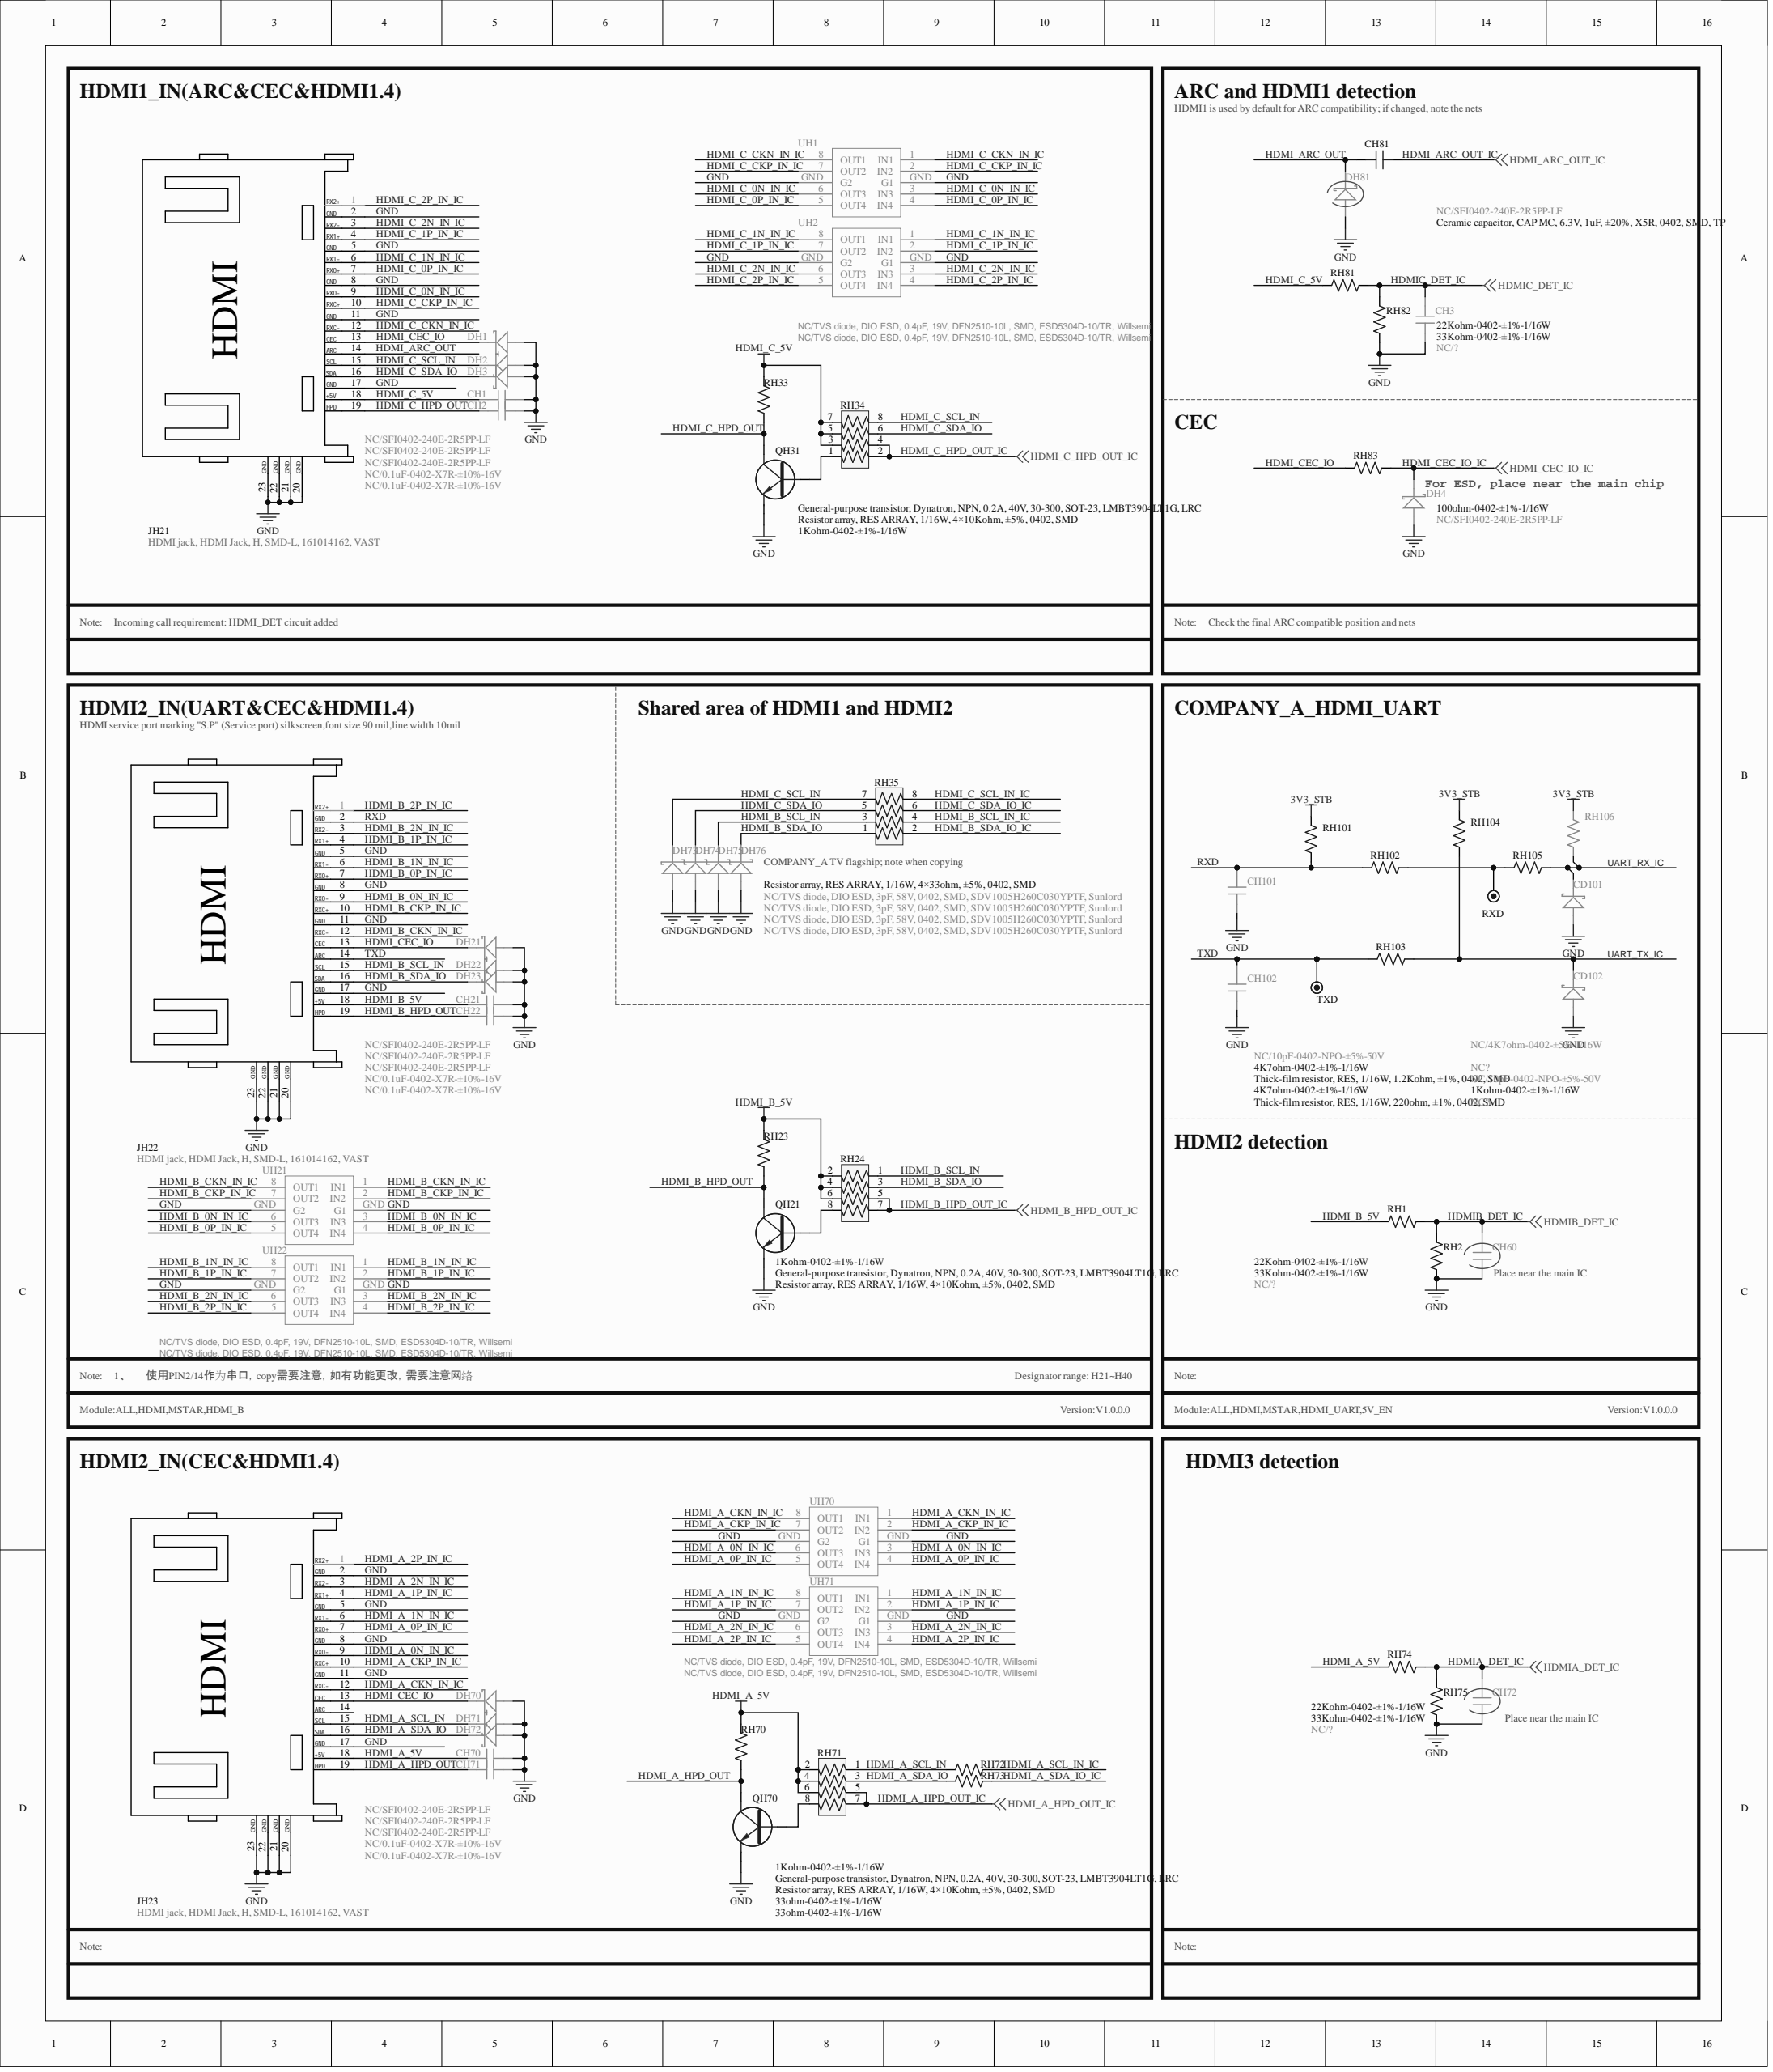Circuit board | Altium Designer | 541 parts | 263 nets | one sheet of the schematic
Parts on this sheet (reference | value | footprint):
CD101 | NC? | DIODE-S0402
CD102 | NC? | DIODE-S0402
CH1 | NC/0.1uF-0402-X7R-±10%-16V | C0402
CH2 | NC/0.1uF-0402-X7R-±10%-16V | C0402
CH3 | NC/? | C0402
CH21 | NC/0.1uF-0402-X7R-±10%-16V | C0402
CH22 | NC/0.1uF-0402-X7R-±10%-16V | C0402
CH60 | NC/? | C0402
CH70 | NC/0.1uF-0402-X7R-±10%-16V | C0402
CH71 | NC/0.1uF-0402-X7R-±10%-16V | C0402
CH72 | NC/? | C0402
CH81 | Ceramic capacitor, CAP MC, 6.3V, 1uF, ±20%, X5R, 0402, SMD, TP | C0402
CH101 | NC/10pF-0402-NPO-±5%-50V | C0402
CH102 | NC/10pF-0402-NPO-±5%-50V | C0402
DH1 | NC/SFI0402-240E-2R5PP-LF | DIODE-S0402
DH2 | NC/SFI0402-240E-2R5PP-LF | DIODE-S0402
DH3 | NC/SFI0402-240E-2R5PP-LF | DIODE-S0402
DH4 | NC/SFI0402-240E-2R5PP-LF | DIODE-S0402
DH21 | NC/SFI0402-240E-2R5PP-LF | DIODE-S0402
DH22 | NC/SFI0402-240E-2R5PP-LF | DIODE-S0402
DH23 | NC/SFI0402-240E-2R5PP-LF | DIODE-S0402
DH70 | NC/SFI0402-240E-2R5PP-LF | DIODE-S0402
DH71 | NC/SFI0402-240E-2R5PP-LF | DIODE-S0402
DH72 | NC/SFI0402-240E-2R5PP-LF | DIODE-S0402
DH73 | NC/TVS diode, DIO ESD, 3pF, 58V, 0402, SMD, SDV1005H260C030YPTF, Sunlord | DIODE-S0402
DH74 | NC/TVS diode, DIO ESD, 3pF, 58V, 0402, SMD, SDV1005H260C030YPTF, Sunlord | DIODE-S0402
DH75 | NC/TVS diode, DIO ESD, 3pF, 58V, 0402, SMD, SDV1005H260C030YPTF, Sunlord | DIODE-S0402
DH76 | NC/TVS diode, DIO ESD, 3pF, 58V, 0402, SMD, SDV1005H260C030YPTF, Sunlord | DIODE-S0402
DH81 | NC/SFI0402-240E-2R5PP-LF | DIODE-S0402
JH21 | HDMI jack, HDMI Jack, H, SMD-L, 161014162, VAST | HDMI-HS-1
JH22 | HDMI jack, HDMI Jack, H, SMD-L, 161014162, VAST | HDMI-HS-1
JH23 | HDMI jack, HDMI Jack, H, SMD-L, 161014162, VAST | HDMI-HS-1
QH21 | General-purpose transistor, Dynatron, NPN, 0.2A, 40V, 30-300, SOT-23, LMBT3904LT1G, LRC | SOT-23
QH31 | General-purpose transistor, Dynatron, NPN, 0.2A, 40V, 30-300, SOT-23, LMBT3904LT1G, LRC | SOT-23
QH70 | General-purpose transistor, Dynatron, NPN, 0.2A, 40V, 30-300, SOT-23, LMBT3904LT1G, LRC | SOT-23
RH1 | 22Kohm-0402-±1%-1/16W | R0402
RH2 | 33Kohm-0402-±1%-1/16W | R0402
RH23 | 1Kohm-0402-±1%-1/16W | R0402
RH24 | Resistor array, RES ARRAY, 1/16W, 4×10Kohm, ±5%, 0402, SMD | RA0402
RH33 | 1Kohm-0402-±1%-1/16W | R0402
RH34 | Resistor array, RES ARRAY, 1/16W, 4×10Kohm, ±5%, 0402, SMD | RA0402
RH35 | Resistor array, RES ARRAY, 1/16W, 4×33ohm, ±5%, 0402, SMD | RA0402
RH70 | 1Kohm-0402-±1%-1/16W | R0402
RH71 | Resistor array, RES ARRAY, 1/16W, 4×10Kohm, ±5%, 0402, SMD | RA0402
RH72 | 33ohm-0402-±1%-1/16W | R0402
RH73 | 33ohm-0402-±1%-1/16W | R0402
RH74 | 22Kohm-0402-±1%-1/16W | R0402
RH75 | 33Kohm-0402-±1%-1/16W | R0402
RH81 | 22Kohm-0402-±1%-1/16W | R0402
RH82 | 33Kohm-0402-±1%-1/16W | R0402
RH83 | 100ohm-0402-±1%-1/16W | R0402
RH101 | 4K7ohm-0402-±1%-1/16W | R0402
RH102 | Thick-film resistor, RES, 1/16W, 1.2Kohm, ±1%, 0402, SMD | R0402
RH103 | 1Kohm-0402-±1%-1/16W | R0402
RH104 | 4K7ohm-0402-±1%-1/16W | R0402
RH105 | Thick-film resistor, RES, 1/16W, 220ohm, ±1%, 0402, SMD | R0402
RH106 | NC/4K7ohm-0402-±5%-1/16W | R0402
RXD | TP
TXD | TP
UH1 | NC/TVS diode, DIO ESD, 0.4pF, 19V, DFN2510-10L, SMD, ESD5304D-10/TR, Willsemi | RCL0524P
UH2 | NC/TVS diode, DIO ESD, 0.4pF, 19V, DFN2510-10L, SMD, ESD5304D-10/TR, Willsemi | RCL0524P
UH21 | NC/TVS diode, DIO ESD, 0.4pF, 19V, DFN2510-10L, SMD, ESD5304D-10/TR, Willsemi | RCL0524P
UH22 | NC/TVS diode, DIO ESD, 0.4pF, 19V, DFN2510-10L, SMD, ESD5304D-10/TR, Willsemi | RCL0524P
UH70 | NC/TVS diode, DIO ESD, 0.4pF, 19V, DFN2510-10L, SMD, ESD5304D-10/TR, Willsemi | RCL0524P
UH71 | NC/TVS diode, DIO ESD, 0.4pF, 19V, DFN2510-10L, SMD, ESD5304D-10/TR, Willsemi | RCL0524P
Nets of these parts (net: part-pin ...):
UART_TX_IC: CD102-K RH103-2 RH104-1
UART_RX_IC: CD101-K RH105-2 RH106-1
TXD: CH102-2 RH103-1 TXD-1 JH22-14
RXD: CH101-2 RH101-1 RH102-1 JH22-2
NetRH102_2: RH102-2 RH105-1 RXD-1
NetQH70_B: QH70-B RH71-8
NetQH31_B: QH31-B RH34-1
NetQH21_B: QH21-B RH24-8
HDMIC_DET_IC: CH3-2 RH81-1 RH82-1
HDMIB_DET_IC: CH60-2 RH1-1 RH2-1
HDMIA_DET_IC: CH72-2 RH74-1 RH75-1
HDMI_CEC_IO_IC: DH4-K RH83-1
HDMI_CEC_IO: DH1-K DH21-K DH70-K RH83-2 JH21-13 JH22-13 JH23-13
HDMI_C_SDA_IO_IC: RH35-6
HDMI_C_SDA_IO: DH3-K DH74-K RH34-6 RH35-5 JH21-16
HDMI_C_SCL_IN_IC: RH35-8
HDMI_C_SCL_IN: DH2-K DH73-K RH34-8 RH35-7 JH21-15
HDMI_C_HPD_OUT_IC: RH34-2 RH34-4
HDMI_C_HPD_OUT: CH2-1 QH31-C RH33-1 JH21-19
HDMI_C_CKP_IN_IC: UH1-2 UH1-7 JH21-10
HDMI_C_CKN_IN_IC: UH1-1 UH1-8 JH21-12
HDMI_C_5V: CH1-1 RH33-2 RH34-3 RH34-5 RH34-7 RH81-2 JH21-18
HDMI_C_2P_IN_IC: UH2-4 UH2-5 JH21-1
HDMI_C_2N_IN_IC: UH2-3 UH2-6 JH21-3
HDMI_C_1P_IN_IC: UH2-2 UH2-7 JH21-4
HDMI_C_1N_IN_IC: UH2-1 UH2-8 JH21-6
HDMI_C_0P_IN_IC: UH1-4 UH1-5 JH21-7
HDMI_C_0N_IN_IC: UH1-3 UH1-6 JH21-9
HDMI_B_SDA_IO_IC: RH35-2
HDMI_B_SDA_IO: DH23-K DH76-K RH24-3 RH35-1 JH22-16
HDMI_B_SCL_IN_IC: RH35-4
HDMI_B_SCL_IN: DH22-K DH75-K RH24-1 RH35-3 JH22-15
HDMI_B_HPD_OUT_IC: RH24-5 RH24-7
HDMI_B_HPD_OUT: CH22-1 QH21-C RH23-1 JH22-19
HDMI_B_CKP_IN_IC: UH21-2 UH21-7 JH22-10
HDMI_B_CKN_IN_IC: UH21-1 UH21-8 JH22-12
HDMI_B_5V: CH21-1 RH1-2 RH23-2 RH24-2 RH24-4 RH24-6 JH22-18
HDMI_B_2P_IN_IC: UH22-4 UH22-5 JH22-1
HDMI_B_2N_IN_IC: UH22-3 UH22-6 JH22-3
HDMI_B_1P_IN_IC: UH22-2 UH22-7 JH22-4
HDMI_B_1N_IN_IC: UH22-1 UH22-8 JH22-6
HDMI_B_0P_IN_IC: UH21-4 UH21-5 JH22-7
HDMI_B_0N_IN_IC: UH21-3 UH21-6 JH22-9
HDMI_ARC_OUT_IC: CH81-2
HDMI_ARC_OUT: CH81-1 DH81-K JH21-14
HDMI_A_SDA_IO_IC: RH73-2
HDMI_A_SDA_IO: DH72-K RH71-3 RH73-1 JH23-16
HDMI_A_SCL_IN_IC: RH72-2
HDMI_A_SCL_IN: DH71-K RH71-1 RH72-1 JH23-15
HDMI_A_HPD_OUT_IC: RH71-5 RH71-7
HDMI_A_HPD_OUT: CH71-1 QH70-C RH70-1 JH23-19
HDMI_A_CKP_IN_IC: UH70-2 UH70-7 JH23-10
HDMI_A_CKN_IN_IC: UH70-1 UH70-8 JH23-12
HDMI_A_5V: CH70-1 RH70-2 RH71-2 RH71-4 RH71-6 RH74-2 JH23-18
HDMI_A_2P_IN_IC: UH71-4 UH71-5 JH23-1
HDMI_A_2N_IN_IC: UH71-3 UH71-6 JH23-3
HDMI_A_1P_IN_IC: UH71-2 UH71-7 JH23-4
HDMI_A_1N_IN_IC: UH71-1 UH71-8 JH23-6
HDMI_A_0P_IN_IC: UH70-4 UH70-5 JH23-7
HDMI_A_0N_IN_IC: UH70-3 UH70-6 JH23-9
GND: CD101-A CD102-A CH1-2 CH2-2 CH3-1 CH21-2 CH22-2 CH60-1 CH70-2 CH71-2 CH72-1 CH101-1 CH102-1 DH1-A DH2-A DH3-A DH4-A DH21-A DH22-A DH23-A DH70-A DH71-A DH72-A DH73-A DH74-A DH75-A DH76-A DH81-A QH21-E QH31-E QH70-E RH2-2 RH75-2 RH82-2 UH1-GND UH2-GND UH21-GND UH22-GND UH70-GND UH71-GND JH21-2 JH21-5 JH21-8 JH21-11 JH21-17 JH21-20 JH21-21 JH21-22 JH21-23 JH22-5 JH22-8 JH22-11 JH22-17 JH22-20 JH22-21 JH22-22 JH22-23 JH23-2 JH23-5 JH23-8 JH23-11 JH23-17 JH23-20 JH23-21 JH23-22 JH23-23
3V3_STB: RH101-2 RH104-2 RH106-2